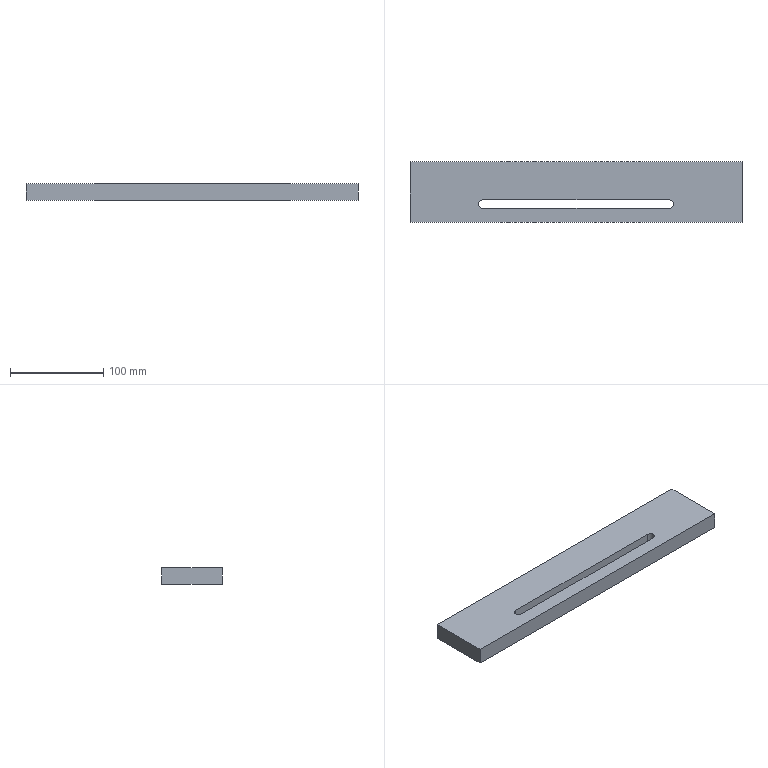Part | STEP file | Superstructure_1 | 1 solid | 10 faces | box 356.5 x 65 x 18 mm | volume 383560 mm3 | plane 8 | cylinder 2 | commonest cylinder face diameters 9 x2
STEP:
#1=CARTESIAN_POINT('',(0.,0.,0.));
#2=DIRECTION('',(0.,0.,1.));
#3=DIRECTION('',(1.,0.,0.));
#4=AXIS2_PLACEMENT_3D('',#1,#2,#3);
#5=CARTESIAN_POINT('',(-178.25,32.5,9.));
#6=VERTEX_POINT('',#5);
#7=CARTESIAN_POINT('',(-178.25,-32.5,9.));
#8=VERTEX_POINT('',#7);
#9=CARTESIAN_POINT('',(-178.25,32.5,9.));
#10=DIRECTION('',(0.,-1.,0.));
#11=VECTOR('',#10,1.);
#12=LINE('',#9,#11);
#13=CARTESIAN_POINT('',(-178.25,32.5,9.));
#14=DIRECTION('',(1.,0.,0.));
#15=DIRECTION('',(0.,0.,-1.));
#16=AXIS2_PLACEMENT_3D('',#13,#14,#15);
#17=PLANE('',#16);
#18=CARTESIAN_POINT('',(0.,0.));
#19=DIRECTION('',(0.,-1.));
#20=VECTOR('',#19,1.);
#21=LINE('',#18,#20);
#22=(GEOMETRIC_REPRESENTATION_CONTEXT(2)PARAMETRIC_REPRESENTATION_CONTEXT()REPRESENTATION_CONTEXT('',''));
#23=DEFINITIONAL_REPRESENTATION('',(#21),#22);
#24=PCURVE('',#17,#23);
#25=CARTESIAN_POINT('',(178.25,32.5,9.));
#26=DIRECTION('',(0.,0.,-1.));
#27=DIRECTION('',(-1.,0.,0.));
#28=AXIS2_PLACEMENT_3D('',#25,#26,#27);
#29=PLANE('',#28);
#30=CARTESIAN_POINT('',(356.5,0.));
#31=DIRECTION('',(0.,-1.));
#32=VECTOR('',#31,1.);
#33=LINE('',#30,#32);
#34=(GEOMETRIC_REPRESENTATION_CONTEXT(2)PARAMETRIC_REPRESENTATION_CONTEXT()REPRESENTATION_CONTEXT('',''));
#35=DEFINITIONAL_REPRESENTATION('',(#33),#34);
#36=PCURVE('',#29,#35);
#37=SURFACE_CURVE('',#12,(#24,#36),.PCURVE_S1.);
#38=EDGE_CURVE('',#6,#8,#37,.T.);
#39=ORIENTED_EDGE('',*,*,#38,.T.);
#40=CARTESIAN_POINT('',(-178.25,-32.5,-9.));
#41=VERTEX_POINT('',#40);
#42=CARTESIAN_POINT('',(-178.25,-32.5,9.));
#43=DIRECTION('',(0.,0.,-1.));
#44=VECTOR('',#43,1.);
#45=LINE('',#42,#44);
#46=CARTESIAN_POINT('',(0.,-65.));
#47=DIRECTION('',(1.,0.));
#48=VECTOR('',#47,1.);
#49=LINE('',#46,#48);
#50=(GEOMETRIC_REPRESENTATION_CONTEXT(2)PARAMETRIC_REPRESENTATION_CONTEXT()REPRESENTATION_CONTEXT('',''));
#51=DEFINITIONAL_REPRESENTATION('',(#49),#50);
#52=PCURVE('',#17,#51);
#53=CARTESIAN_POINT('',(0.,-32.5,0.));
#54=DIRECTION('',(0.,1.,0.));
#55=DIRECTION('',(0.,0.,1.));
#56=AXIS2_PLACEMENT_3D('',#53,#54,#55);
#57=PLANE('',#56);
#58=CARTESIAN_POINT('',(9.,-178.25));
#59=DIRECTION('',(-1.,0.));
#60=VECTOR('',#59,1.);
#61=LINE('',#58,#60);
#62=(GEOMETRIC_REPRESENTATION_CONTEXT(2)PARAMETRIC_REPRESENTATION_CONTEXT()REPRESENTATION_CONTEXT('',''));
#63=DEFINITIONAL_REPRESENTATION('',(#61),#62);
#64=PCURVE('',#57,#63);
#65=SURFACE_CURVE('',#45,(#52,#64),.PCURVE_S1.);
#66=EDGE_CURVE('',#8,#41,#65,.T.);
#67=ORIENTED_EDGE('',*,*,#66,.T.);
#68=CARTESIAN_POINT('',(-178.25,32.5,-9.));
#69=VERTEX_POINT('',#68);
#70=CARTESIAN_POINT('',(-178.25,32.5,-9.));
#71=DIRECTION('',(0.,-1.,0.));
#72=VECTOR('',#71,1.);
#73=LINE('',#70,#72);
#74=CARTESIAN_POINT('',(18.,0.));
#75=DIRECTION('',(0.,-1.));
#76=VECTOR('',#75,1.);
#77=LINE('',#74,#76);
#78=(GEOMETRIC_REPRESENTATION_CONTEXT(2)PARAMETRIC_REPRESENTATION_CONTEXT()REPRESENTATION_CONTEXT('',''));
#79=DEFINITIONAL_REPRESENTATION('',(#77),#78);
#80=PCURVE('',#17,#79);
#81=CARTESIAN_POINT('',(-178.25,32.5,-9.));
#82=DIRECTION('',(0.,0.,1.));
#83=DIRECTION('',(1.,0.,0.));
#84=AXIS2_PLACEMENT_3D('',#81,#82,#83);
#85=PLANE('',#84);
#86=CARTESIAN_POINT('',(0.,0.));
#87=DIRECTION('',(0.,-1.));
#88=VECTOR('',#87,1.);
#89=LINE('',#86,#88);
#90=(GEOMETRIC_REPRESENTATION_CONTEXT(2)PARAMETRIC_REPRESENTATION_CONTEXT()REPRESENTATION_CONTEXT('',''));
#91=DEFINITIONAL_REPRESENTATION('',(#89),#90);
#92=PCURVE('',#85,#91);
#93=SURFACE_CURVE('',#73,(#80,#92),.PCURVE_S1.);
#94=EDGE_CURVE('',#69,#41,#93,.T.);
#95=ORIENTED_EDGE('',*,*,#94,.F.);
#96=CARTESIAN_POINT('',(-178.25,32.5,9.));
#97=DIRECTION('',(0.,0.,-1.));
#98=VECTOR('',#97,1.);
#99=LINE('',#96,#98);
#100=CARTESIAN_POINT('',(0.,0.));
#101=DIRECTION('',(1.,0.));
#102=VECTOR('',#101,1.);
#103=LINE('',#100,#102);
#104=(GEOMETRIC_REPRESENTATION_CONTEXT(2)PARAMETRIC_REPRESENTATION_CONTEXT()REPRESENTATION_CONTEXT('',''));
#105=DEFINITIONAL_REPRESENTATION('',(#103),#104);
#106=PCURVE('',#17,#105);
#107=CARTESIAN_POINT('',(0.,32.5,0.));
#108=DIRECTION('',(0.,1.,0.));
#109=DIRECTION('',(0.,0.,1.));
#110=AXIS2_PLACEMENT_3D('',#107,#108,#109);
#111=PLANE('',#110);
#112=CARTESIAN_POINT('',(9.,-178.25));
#113=DIRECTION('',(-1.,0.));
#114=VECTOR('',#113,1.);
#115=LINE('',#112,#114);
#116=(GEOMETRIC_REPRESENTATION_CONTEXT(2)PARAMETRIC_REPRESENTATION_CONTEXT()REPRESENTATION_CONTEXT('',''));
#117=DEFINITIONAL_REPRESENTATION('',(#115),#116);
#118=PCURVE('',#111,#117);
#119=SURFACE_CURVE('',#99,(#106,#118),.PCURVE_S1.);
#120=EDGE_CURVE('',#6,#69,#119,.T.);
#121=ORIENTED_EDGE('',*,*,#120,.F.);
#122=EDGE_LOOP('',(#39,#67,#95,#121));
#123=FACE_BOUND('',#122,.F.);
#124=ADVANCED_FACE('',(#123),#17,.F.);
#125=CARTESIAN_POINT('',(178.25,32.5,9.));
#126=VERTEX_POINT('',#125);
#127=CARTESIAN_POINT('',(178.25,-32.5,9.));
#128=VERTEX_POINT('',#127);
#129=CARTESIAN_POINT('',(178.25,32.5,9.));
#130=DIRECTION('',(0.,-1.,0.));
#131=VECTOR('',#130,1.);
#132=LINE('',#129,#131);
#133=CARTESIAN_POINT('',(0.,0.));
#134=DIRECTION('',(0.,-1.));
#135=VECTOR('',#134,1.);
#136=LINE('',#133,#135);
#137=(GEOMETRIC_REPRESENTATION_CONTEXT(2)PARAMETRIC_REPRESENTATION_CONTEXT()REPRESENTATION_CONTEXT('',''));
#138=DEFINITIONAL_REPRESENTATION('',(#136),#137);
#139=PCURVE('',#29,#138);
#140=CARTESIAN_POINT('',(178.25,32.5,-9.));
#141=DIRECTION('',(-1.,0.,0.));
#142=DIRECTION('',(0.,0.,1.));
#143=AXIS2_PLACEMENT_3D('',#140,#141,#142);
#144=PLANE('',#143);
#145=CARTESIAN_POINT('',(18.,0.));
#146=DIRECTION('',(0.,-1.));
#147=VECTOR('',#146,1.);
#148=LINE('',#145,#147);
#149=(GEOMETRIC_REPRESENTATION_CONTEXT(2)PARAMETRIC_REPRESENTATION_CONTEXT()REPRESENTATION_CONTEXT('',''));
#150=DEFINITIONAL_REPRESENTATION('',(#148),#149);
#151=PCURVE('',#144,#150);
#152=SURFACE_CURVE('',#132,(#139,#151),.PCURVE_S1.);
#153=EDGE_CURVE('',#126,#128,#152,.T.);
#154=ORIENTED_EDGE('',*,*,#153,.T.);
#155=CARTESIAN_POINT('',(178.25,-32.5,9.));
#156=DIRECTION('',(-1.,0.,0.));
#157=VECTOR('',#156,1.);
#158=LINE('',#155,#157);
#159=CARTESIAN_POINT('',(0.,-65.));
#160=DIRECTION('',(1.,0.));
#161=VECTOR('',#160,1.);
#162=LINE('',#159,#161);
#163=(GEOMETRIC_REPRESENTATION_CONTEXT(2)PARAMETRIC_REPRESENTATION_CONTEXT()REPRESENTATION_CONTEXT('',''));
#164=DEFINITIONAL_REPRESENTATION('',(#162),#163);
#165=PCURVE('',#29,#164);
#166=CARTESIAN_POINT('',(9.,178.25));
#167=DIRECTION('',(0.,-1.));
#168=VECTOR('',#167,1.);
#169=LINE('',#166,#168);
#170=(GEOMETRIC_REPRESENTATION_CONTEXT(2)PARAMETRIC_REPRESENTATION_CONTEXT()REPRESENTATION_CONTEXT('',''));
#171=DEFINITIONAL_REPRESENTATION('',(#169),#170);
#172=PCURVE('',#57,#171);
#173=SURFACE_CURVE('',#158,(#165,#172),.PCURVE_S1.);
#174=EDGE_CURVE('',#128,#8,#173,.T.);
#175=ORIENTED_EDGE('',*,*,#174,.T.);
#176=ORIENTED_EDGE('',*,*,#38,.F.);
#177=CARTESIAN_POINT('',(178.25,32.5,9.));
#178=DIRECTION('',(-1.,0.,0.));
#179=VECTOR('',#178,1.);
#180=LINE('',#177,#179);
#181=CARTESIAN_POINT('',(0.,0.));
#182=DIRECTION('',(1.,0.));
#183=VECTOR('',#182,1.);
#184=LINE('',#181,#183);
#185=(GEOMETRIC_REPRESENTATION_CONTEXT(2)PARAMETRIC_REPRESENTATION_CONTEXT()REPRESENTATION_CONTEXT('',''));
#186=DEFINITIONAL_REPRESENTATION('',(#184),#185);
#187=PCURVE('',#29,#186);
#188=CARTESIAN_POINT('',(9.,178.25));
#189=DIRECTION('',(0.,-1.));
#190=VECTOR('',#189,1.);
#191=LINE('',#188,#190);
#192=(GEOMETRIC_REPRESENTATION_CONTEXT(2)PARAMETRIC_REPRESENTATION_CONTEXT()REPRESENTATION_CONTEXT('',''));
#193=DEFINITIONAL_REPRESENTATION('',(#191),#192);
#194=PCURVE('',#111,#193);
#195=SURFACE_CURVE('',#180,(#187,#194),.PCURVE_S1.);
#196=EDGE_CURVE('',#126,#6,#195,.T.);
#197=ORIENTED_EDGE('',*,*,#196,.F.);
#198=EDGE_LOOP('',(#154,#175,#176,#197));
#199=FACE_BOUND('',#198,.F.);
#200=CARTESIAN_POINT('',(100.,-8.5,9.));
#201=VERTEX_POINT('',#200);
#202=CARTESIAN_POINT('',(-100.,-8.5,9.));
#203=VERTEX_POINT('',#202);
#204=CARTESIAN_POINT('',(39.125,-8.5,9.));
#205=DIRECTION('',(-1.,0.,0.));
#206=VECTOR('',#205,1.);
#207=LINE('',#204,#206);
#208=CARTESIAN_POINT('',(139.125,-41.));
#209=DIRECTION('',(1.,0.));
#210=VECTOR('',#209,1.);
#211=LINE('',#208,#210);
#212=(GEOMETRIC_REPRESENTATION_CONTEXT(2)PARAMETRIC_REPRESENTATION_CONTEXT()REPRESENTATION_CONTEXT('',''));
#213=DEFINITIONAL_REPRESENTATION('',(#211),#212);
#214=PCURVE('',#29,#213);
#215=CARTESIAN_POINT('',(-100.,-8.5,15.));
#216=DIRECTION('',(0.,-1.,0.));
#217=DIRECTION('',(1.,0.,0.));
#218=AXIS2_PLACEMENT_3D('',#215,#216,#217);
#219=PLANE('',#218);
#220=CARTESIAN_POINT('',(139.125,-6.));
#221=DIRECTION('',(-1.,0.));
#222=VECTOR('',#221,1.);
#223=LINE('',#220,#222);
#224=(GEOMETRIC_REPRESENTATION_CONTEXT(2)PARAMETRIC_REPRESENTATION_CONTEXT()REPRESENTATION_CONTEXT('',''));
#225=DEFINITIONAL_REPRESENTATION('',(#223),#224);
#226=PCURVE('',#219,#225);
#227=SURFACE_CURVE('',#207,(#214,#226),.PCURVE_S1.);
#228=EDGE_CURVE('',#201,#203,#227,.T.);
#229=ORIENTED_EDGE('',*,*,#228,.T.);
#230=CARTESIAN_POINT('',(-100.,-17.5,9.));
#231=VERTEX_POINT('',#230);
#232=CARTESIAN_POINT('',(-100.,-13.,9.));
#233=DIRECTION('',(0.,0.,1.));
#234=DIRECTION('',(1.,0.,0.));
#235=AXIS2_PLACEMENT_3D('',#232,#233,#234);
#236=CIRCLE('',#235,4.5);
#237=CARTESIAN_POINT('',(273.75,-45.5));
#238=CARTESIAN_POINT('',(273.75,-37.706));
#239=CARTESIAN_POINT('',(280.5,-41.603));
#240=CARTESIAN_POINT('',(287.25,-45.5));
#241=CARTESIAN_POINT('',(280.5,-49.397));
#242=CARTESIAN_POINT('',(273.75,-53.294));
#243=CARTESIAN_POINT('',(273.75,-45.5));
#244=(BOUNDED_CURVE()B_SPLINE_CURVE(2,(#237,#238,#239,#240,#241,#242,#243),.UNSPECIFIED.,.T.,.F.)B_SPLINE_CURVE_WITH_KNOTS((1,2,2,2,2,1),(-2.094,0.,2.094,4.189,6.283,8.378),.UNSPECIFIED.)CURVE()GEOMETRIC_REPRESENTATION_ITEM()RATIONAL_B_SPLINE_CURVE((1.,0.5,1.,0.5,1.,0.5,1.))REPRESENTATION_ITEM(''));
#245=(GEOMETRIC_REPRESENTATION_CONTEXT(2)PARAMETRIC_REPRESENTATION_CONTEXT()REPRESENTATION_CONTEXT('',''));
#246=DEFINITIONAL_REPRESENTATION('',(#244),#245);
#247=PCURVE('',#29,#246);
#248=CARTESIAN_POINT('',(-100.,-13.,15.));
#249=DIRECTION('',(0.,0.,1.));
#250=DIRECTION('',(1.,0.,0.));
#251=AXIS2_PLACEMENT_3D('',#248,#249,#250);
#252=CYLINDRICAL_SURFACE('',#251,4.5);
#253=CARTESIAN_POINT('',(0.,-6.));
#254=DIRECTION('',(1.,0.));
#255=VECTOR('',#254,1.);
#256=LINE('',#253,#255);
#257=(GEOMETRIC_REPRESENTATION_CONTEXT(2)PARAMETRIC_REPRESENTATION_CONTEXT()REPRESENTATION_CONTEXT('',''));
#258=DEFINITIONAL_REPRESENTATION('',(#256),#257);
#259=PCURVE('',#252,#258);
#260=SURFACE_CURVE('',#236,(#247,#259),.PCURVE_S1.);
#261=EDGE_CURVE('',#203,#231,#260,.T.);
#262=ORIENTED_EDGE('',*,*,#261,.T.);
#263=CARTESIAN_POINT('',(100.,-17.5,9.));
#264=VERTEX_POINT('',#263);
#265=CARTESIAN_POINT('',(39.125,-17.5,9.));
#266=DIRECTION('',(-1.,0.,0.));
#267=VECTOR('',#266,1.);
#268=LINE('',#265,#267);
#269=CARTESIAN_POINT('',(139.125,-50.));
#270=DIRECTION('',(1.,0.));
#271=VECTOR('',#270,1.);
#272=LINE('',#269,#271);
#273=(GEOMETRIC_REPRESENTATION_CONTEXT(2)PARAMETRIC_REPRESENTATION_CONTEXT()REPRESENTATION_CONTEXT('',''));
#274=DEFINITIONAL_REPRESENTATION('',(#272),#273);
#275=PCURVE('',#29,#274);
#276=CARTESIAN_POINT('',(-100.,-17.5,15.));
#277=DIRECTION('',(0.,-1.,0.));
#278=DIRECTION('',(1.,0.,0.));
#279=AXIS2_PLACEMENT_3D('',#276,#277,#278);
#280=PLANE('',#279);
#281=CARTESIAN_POINT('',(139.125,-6.));
#282=DIRECTION('',(-1.,0.));
#283=VECTOR('',#282,1.);
#284=LINE('',#281,#283);
#285=(GEOMETRIC_REPRESENTATION_CONTEXT(2)PARAMETRIC_REPRESENTATION_CONTEXT()REPRESENTATION_CONTEXT('',''));
#286=DEFINITIONAL_REPRESENTATION('',(#284),#285);
#287=PCURVE('',#280,#286);
#288=SURFACE_CURVE('',#268,(#275,#287),.PCURVE_S1.);
#289=EDGE_CURVE('',#264,#231,#288,.T.);
#290=ORIENTED_EDGE('',*,*,#289,.F.);
#291=CARTESIAN_POINT('',(100.,-13.,9.));
#292=DIRECTION('',(0.,0.,1.));
#293=DIRECTION('',(1.,0.,0.));
#294=AXIS2_PLACEMENT_3D('',#291,#292,#293);
#295=CIRCLE('',#294,4.5);
#296=CARTESIAN_POINT('',(73.75,-45.5));
#297=CARTESIAN_POINT('',(73.75,-37.706));
#298=CARTESIAN_POINT('',(80.5,-41.603));
#299=CARTESIAN_POINT('',(87.25,-45.5));
#300=CARTESIAN_POINT('',(80.5,-49.397));
#301=CARTESIAN_POINT('',(73.75,-53.294));
#302=CARTESIAN_POINT('',(73.75,-45.5));
#303=(BOUNDED_CURVE()B_SPLINE_CURVE(2,(#296,#297,#298,#299,#300,#301,#302),.UNSPECIFIED.,.T.,.F.)B_SPLINE_CURVE_WITH_KNOTS((1,2,2,2,2,1),(-2.094,0.,2.094,4.189,6.283,8.378),.UNSPECIFIED.)CURVE()GEOMETRIC_REPRESENTATION_ITEM()RATIONAL_B_SPLINE_CURVE((1.,0.5,1.,0.5,1.,0.5,1.))REPRESENTATION_ITEM(''));
#304=(GEOMETRIC_REPRESENTATION_CONTEXT(2)PARAMETRIC_REPRESENTATION_CONTEXT()REPRESENTATION_CONTEXT('',''));
#305=DEFINITIONAL_REPRESENTATION('',(#303),#304);
#306=PCURVE('',#29,#305);
#307=CARTESIAN_POINT('',(100.,-13.,15.));
#308=DIRECTION('',(0.,0.,1.));
#309=DIRECTION('',(1.,0.,0.));
#310=AXIS2_PLACEMENT_3D('',#307,#308,#309);
#311=CYLINDRICAL_SURFACE('',#310,4.5);
#312=CARTESIAN_POINT('',(0.,-6.));
#313=DIRECTION('',(1.,0.));
#314=VECTOR('',#313,1.);
#315=LINE('',#312,#314);
#316=(GEOMETRIC_REPRESENTATION_CONTEXT(2)PARAMETRIC_REPRESENTATION_CONTEXT()REPRESENTATION_CONTEXT('',''));
#317=DEFINITIONAL_REPRESENTATION('',(#315),#316);
#318=PCURVE('',#311,#317);
#319=SURFACE_CURVE('',#295,(#306,#318),.PCURVE_S1.);
#320=EDGE_CURVE('',#264,#201,#319,.T.);
#321=ORIENTED_EDGE('',*,*,#320,.T.);
#322=EDGE_LOOP('',(#229,#262,#290,#321));
#323=FACE_BOUND('',#322,.F.);
#324=ADVANCED_FACE('',(#199,#323),#29,.F.);
#325=ORIENTED_EDGE('',*,*,#94,.T.);
#326=CARTESIAN_POINT('',(178.25,-32.5,-9.));
#327=VERTEX_POINT('',#326);
#328=CARTESIAN_POINT('',(-178.25,-32.5,-9.));
#329=DIRECTION('',(1.,0.,0.));
#330=VECTOR('',#329,1.);
#331=LINE('',#328,#330);
#332=CARTESIAN_POINT('',(0.,-65.));
#333=DIRECTION('',(1.,0.));
#334=VECTOR('',#333,1.);
#335=LINE('',#332,#334);
#336=(GEOMETRIC_REPRESENTATION_CONTEXT(2)PARAMETRIC_REPRESENTATION_CONTEXT()REPRESENTATION_CONTEXT('',''));
#337=DEFINITIONAL_REPRESENTATION('',(#335),#336);
#338=PCURVE('',#85,#337);
#339=CARTESIAN_POINT('',(-9.,-178.25));
#340=DIRECTION('',(0.,1.));
#341=VECTOR('',#340,1.);
#342=LINE('',#339,#341);
#343=(GEOMETRIC_REPRESENTATION_CONTEXT(2)PARAMETRIC_REPRESENTATION_CONTEXT()REPRESENTATION_CONTEXT('',''));
#344=DEFINITIONAL_REPRESENTATION('',(#342),#343);
#345=PCURVE('',#57,#344);
#346=SURFACE_CURVE('',#331,(#338,#345),.PCURVE_S1.);
#347=EDGE_CURVE('',#41,#327,#346,.T.);
#348=ORIENTED_EDGE('',*,*,#347,.T.);
#349=CARTESIAN_POINT('',(178.25,32.5,-9.));
#350=VERTEX_POINT('',#349);
#351=CARTESIAN_POINT('',(178.25,32.5,-9.));
#352=DIRECTION('',(0.,-1.,0.));
#353=VECTOR('',#352,1.);
#354=LINE('',#351,#353);
#355=CARTESIAN_POINT('',(356.5,0.));
#356=DIRECTION('',(0.,-1.));
#357=VECTOR('',#356,1.);
#358=LINE('',#355,#357);
#359=(GEOMETRIC_REPRESENTATION_CONTEXT(2)PARAMETRIC_REPRESENTATION_CONTEXT()REPRESENTATION_CONTEXT('',''));
#360=DEFINITIONAL_REPRESENTATION('',(#358),#359);
#361=PCURVE('',#85,#360);
#362=CARTESIAN_POINT('',(0.,0.));
#363=DIRECTION('',(0.,-1.));
#364=VECTOR('',#363,1.);
#365=LINE('',#362,#364);
#366=(GEOMETRIC_REPRESENTATION_CONTEXT(2)PARAMETRIC_REPRESENTATION_CONTEXT()REPRESENTATION_CONTEXT('',''));
#367=DEFINITIONAL_REPRESENTATION('',(#365),#366);
#368=PCURVE('',#144,#367);
#369=SURFACE_CURVE('',#354,(#361,#368),.PCURVE_S1.);
#370=EDGE_CURVE('',#350,#327,#369,.T.);
#371=ORIENTED_EDGE('',*,*,#370,.F.);
#372=CARTESIAN_POINT('',(-178.25,32.5,-9.));
#373=DIRECTION('',(1.,0.,0.));
#374=VECTOR('',#373,1.);
#375=LINE('',#372,#374);
#376=CARTESIAN_POINT('',(0.,0.));
#377=DIRECTION('',(1.,0.));
#378=VECTOR('',#377,1.);
#379=LINE('',#376,#378);
#380=(GEOMETRIC_REPRESENTATION_CONTEXT(2)PARAMETRIC_REPRESENTATION_CONTEXT()REPRESENTATION_CONTEXT('',''));
#381=DEFINITIONAL_REPRESENTATION('',(#379),#380);
#382=PCURVE('',#85,#381);
#383=CARTESIAN_POINT('',(-9.,-178.25));
#384=DIRECTION('',(0.,1.));
#385=VECTOR('',#384,1.);
#386=LINE('',#383,#385);
#387=(GEOMETRIC_REPRESENTATION_CONTEXT(2)PARAMETRIC_REPRESENTATION_CONTEXT()REPRESENTATION_CONTEXT('',''));
#388=DEFINITIONAL_REPRESENTATION('',(#386),#387);
#389=PCURVE('',#111,#388);
#390=SURFACE_CURVE('',#375,(#382,#389),.PCURVE_S1.);
#391=EDGE_CURVE('',#69,#350,#390,.T.);
#392=ORIENTED_EDGE('',*,*,#391,.F.);
#393=EDGE_LOOP('',(#325,#348,#371,#392));
#394=FACE_BOUND('',#393,.F.);
#395=CARTESIAN_POINT('',(-100.,-8.5,-9.));
#396=VERTEX_POINT('',#395);
#397=CARTESIAN_POINT('',(-100.,-17.5,-9.));
#398=VERTEX_POINT('',#397);
#399=CARTESIAN_POINT('',(-100.,-13.,-9.));
#400=DIRECTION('',(0.,0.,1.));
#401=DIRECTION('',(1.,0.,0.));
#402=AXIS2_PLACEMENT_3D('',#399,#400,#401);
#403=CIRCLE('',#402,4.5);
#404=CARTESIAN_POINT('',(78.25,-45.5));
#405=DIRECTION('',(1.,0.));
#406=AXIS2_PLACEMENT_2D('',#404,#405);
#407=CIRCLE('',#406,4.5);
#408=(GEOMETRIC_REPRESENTATION_CONTEXT(2)PARAMETRIC_REPRESENTATION_CONTEXT()REPRESENTATION_CONTEXT('',''));
#409=DEFINITIONAL_REPRESENTATION('',(#407),#408);
#410=PCURVE('',#85,#409);
#411=CARTESIAN_POINT('',(0.,-24.));
#412=DIRECTION('',(1.,0.));
#413=VECTOR('',#412,1.);
#414=LINE('',#411,#413);
#415=(GEOMETRIC_REPRESENTATION_CONTEXT(2)PARAMETRIC_REPRESENTATION_CONTEXT()REPRESENTATION_CONTEXT('',''));
#416=DEFINITIONAL_REPRESENTATION('',(#414),#415);
#417=PCURVE('',#252,#416);
#418=SURFACE_CURVE('',#403,(#410,#417),.PCURVE_S1.);
#419=EDGE_CURVE('',#396,#398,#418,.T.);
#420=ORIENTED_EDGE('',*,*,#419,.F.);
#421=CARTESIAN_POINT('',(100.,-8.5,-9.));
#422=VERTEX_POINT('',#421);
#423=CARTESIAN_POINT('',(-139.125,-8.5,-9.));
#424=DIRECTION('',(1.,0.,0.));
#425=VECTOR('',#424,1.);
#426=LINE('',#423,#425);
#427=CARTESIAN_POINT('',(39.125,-41.));
#428=DIRECTION('',(1.,0.));
#429=VECTOR('',#428,1.);
#430=LINE('',#427,#429);
#431=(GEOMETRIC_REPRESENTATION_CONTEXT(2)PARAMETRIC_REPRESENTATION_CONTEXT()REPRESENTATION_CONTEXT('',''));
#432=DEFINITIONAL_REPRESENTATION('',(#430),#431);
#433=PCURVE('',#85,#432);
#434=CARTESIAN_POINT('',(-39.125,-24.));
#435=DIRECTION('',(1.,0.));
#436=VECTOR('',#435,1.);
#437=LINE('',#434,#436);
#438=(GEOMETRIC_REPRESENTATION_CONTEXT(2)PARAMETRIC_REPRESENTATION_CONTEXT()REPRESENTATION_CONTEXT('',''));
#439=DEFINITIONAL_REPRESENTATION('',(#437),#438);
#440=PCURVE('',#219,#439);
#441=SURFACE_CURVE('',#426,(#433,#440),.PCURVE_S1.);
#442=EDGE_CURVE('',#396,#422,#441,.T.);
#443=ORIENTED_EDGE('',*,*,#442,.T.);
#444=CARTESIAN_POINT('',(100.,-17.5,-9.));
#445=VERTEX_POINT('',#444);
#446=CARTESIAN_POINT('',(100.,-13.,-9.));
#447=DIRECTION('',(0.,0.,1.));
#448=DIRECTION('',(1.,0.,0.));
#449=AXIS2_PLACEMENT_3D('',#446,#447,#448);
#450=CIRCLE('',#449,4.5);
#451=CARTESIAN_POINT('',(278.25,-45.5));
#452=DIRECTION('',(1.,0.));
#453=AXIS2_PLACEMENT_2D('',#451,#452);
#454=CIRCLE('',#453,4.5);
#455=(GEOMETRIC_REPRESENTATION_CONTEXT(2)PARAMETRIC_REPRESENTATION_CONTEXT()REPRESENTATION_CONTEXT('',''));
#456=DEFINITIONAL_REPRESENTATION('',(#454),#455);
#457=PCURVE('',#85,#456);
#458=CARTESIAN_POINT('',(0.,-24.));
#459=DIRECTION('',(1.,0.));
#460=VECTOR('',#459,1.);
#461=LINE('',#458,#460);
#462=(GEOMETRIC_REPRESENTATION_CONTEXT(2)PARAMETRIC_REPRESENTATION_CONTEXT()REPRESENTATION_CONTEXT('',''));
#463=DEFINITIONAL_REPRESENTATION('',(#461),#462);
#464=PCURVE('',#311,#463);
#465=SURFACE_CURVE('',#450,(#457,#464),.PCURVE_S1.);
#466=EDGE_CURVE('',#445,#422,#465,.T.);
#467=ORIENTED_EDGE('',*,*,#466,.F.);
#468=CARTESIAN_POINT('',(-139.125,-17.5,-9.));
#469=DIRECTION('',(1.,0.,0.));
#470=VECTOR('',#469,1.);
#471=LINE('',#468,#470);
#472=CARTESIAN_POINT('',(39.125,-50.));
#473=DIRECTION('',(1.,0.));
#474=VECTOR('',#473,1.);
#475=LINE('',#472,#474);
#476=(GEOMETRIC_REPRESENTATION_CONTEXT(2)PARAMETRIC_REPRESENTATION_CONTEXT()REPRESENTATION_CONTEXT('',''));
#477=DEFINITIONAL_REPRESENTATION('',(#475),#476);
#478=PCURVE('',#85,#477);
#479=CARTESIAN_POINT('',(-39.125,-24.));
#480=DIRECTION('',(1.,0.));
#481=VECTOR('',#480,1.);
#482=LINE('',#479,#481);
#483=(GEOMETRIC_REPRESENTATION_CONTEXT(2)PARAMETRIC_REPRESENTATION_CONTEXT()REPRESENTATION_CONTEXT('',''));
#484=DEFINITIONAL_REPRESENTATION('',(#482),#483);
#485=PCURVE('',#280,#484);
#486=SURFACE_CURVE('',#471,(#478,#485),.PCURVE_S1.);
#487=EDGE_CURVE('',#398,#445,#486,.T.);
#488=ORIENTED_EDGE('',*,*,#487,.F.);
#489=EDGE_LOOP('',(#420,#443,#467,#488));
#490=FACE_BOUND('',#489,.F.);
#491=ADVANCED_FACE('',(#394,#490),#85,.F.);
#492=ORIENTED_EDGE('',*,*,#120,.T.);
#493=ORIENTED_EDGE('',*,*,#391,.T.);
#494=CARTESIAN_POINT('',(178.25,32.5,-9.));
#495=DIRECTION('',(0.,0.,1.));
#496=VECTOR('',#495,1.);
#497=LINE('',#494,#496);
#498=CARTESIAN_POINT('',(-9.,178.25));
#499=DIRECTION('',(1.,0.));
#500=VECTOR('',#499,1.);
#501=LINE('',#498,#500);
#502=(GEOMETRIC_REPRESENTATION_CONTEXT(2)PARAMETRIC_REPRESENTATION_CONTEXT()REPRESENTATION_CONTEXT('',''));
#503=DEFINITIONAL_REPRESENTATION('',(#501),#502);
#504=PCURVE('',#111,#503);
#505=CARTESIAN_POINT('',(0.,0.));
#506=DIRECTION('',(1.,0.));
#507=VECTOR('',#506,1.);
#508=LINE('',#505,#507);
#509=(GEOMETRIC_REPRESENTATION_CONTEXT(2)PARAMETRIC_REPRESENTATION_CONTEXT()REPRESENTATION_CONTEXT('',''));
#510=DEFINITIONAL_REPRESENTATION('',(#508),#509);
#511=PCURVE('',#144,#510);
#512=SURFACE_CURVE('',#497,(#504,#511),.PCURVE_S1.);
#513=EDGE_CURVE('',#350,#126,#512,.T.);
#514=ORIENTED_EDGE('',*,*,#513,.T.);
#515=ORIENTED_EDGE('',*,*,#196,.T.);
#516=EDGE_LOOP('',(#492,#493,#514,#515));
#517=FACE_BOUND('',#516,.F.);
#518=ADVANCED_FACE('',(#517),#111,.T.);
#519=ORIENTED_EDGE('',*,*,#66,.T.);
#520=ORIENTED_EDGE('',*,*,#347,.T.);
#521=CARTESIAN_POINT('',(178.25,-32.5,-9.));
#522=DIRECTION('',(0.,0.,1.));
#523=VECTOR('',#522,1.);
#524=LINE('',#521,#523);
#525=CARTESIAN_POINT('',(-9.,178.25));
#526=DIRECTION('',(1.,0.));
#527=VECTOR('',#526,1.);
#528=LINE('',#525,#527);
#529=(GEOMETRIC_REPRESENTATION_CONTEXT(2)PARAMETRIC_REPRESENTATION_CONTEXT()REPRESENTATION_CONTEXT('',''));
#530=DEFINITIONAL_REPRESENTATION('',(#528),#529);
#531=PCURVE('',#57,#530);
#532=CARTESIAN_POINT('',(0.,-65.));
#533=DIRECTION('',(1.,0.));
#534=VECTOR('',#533,1.);
#535=LINE('',#532,#534);
#536=(GEOMETRIC_REPRESENTATION_CONTEXT(2)PARAMETRIC_REPRESENTATION_CONTEXT()REPRESENTATION_CONTEXT('',''));
#537=DEFINITIONAL_REPRESENTATION('',(#535),#536);
#538=PCURVE('',#144,#537);
#539=SURFACE_CURVE('',#524,(#531,#538),.PCURVE_S1.);
#540=EDGE_CURVE('',#327,#128,#539,.T.);
#541=ORIENTED_EDGE('',*,*,#540,.T.);
#542=ORIENTED_EDGE('',*,*,#174,.T.);
#543=EDGE_LOOP('',(#519,#520,#541,#542));
#544=FACE_BOUND('',#543,.T.);
#545=ADVANCED_FACE('',(#544),#57,.F.);
#546=ORIENTED_EDGE('',*,*,#370,.T.);
#547=ORIENTED_EDGE('',*,*,#540,.T.);
#548=ORIENTED_EDGE('',*,*,#153,.F.);
#549=ORIENTED_EDGE('',*,*,#513,.F.);
#550=EDGE_LOOP('',(#546,#547,#548,#549));
#551=FACE_BOUND('',#550,.F.);
#552=ADVANCED_FACE('',(#551),#144,.F.);
#553=ORIENTED_EDGE('',*,*,#228,.T.);
#554=CARTESIAN_POINT('',(-100.,-8.5,15.));
#555=DIRECTION('',(0.,0.,-1.));
#556=VECTOR('',#555,1.);
#557=LINE('',#554,#556);
#558=CARTESIAN_POINT('',(0.,0.));
#559=DIRECTION('',(0.,-1.));
#560=VECTOR('',#559,1.);
#561=LINE('',#558,#560);
#562=(GEOMETRIC_REPRESENTATION_CONTEXT(2)PARAMETRIC_REPRESENTATION_CONTEXT()REPRESENTATION_CONTEXT('',''));
#563=DEFINITIONAL_REPRESENTATION('',(#561),#562);
#564=PCURVE('',#219,#563);
#565=CARTESIAN_POINT('',(1.571,0.));
#566=DIRECTION('',(0.,-1.));
#567=VECTOR('',#566,1.);
#568=LINE('',#565,#567);
#569=(GEOMETRIC_REPRESENTATION_CONTEXT(2)PARAMETRIC_REPRESENTATION_CONTEXT()REPRESENTATION_CONTEXT('',''));
#570=DEFINITIONAL_REPRESENTATION('',(#568),#569);
#571=PCURVE('',#252,#570);
#572=SURFACE_CURVE('',#557,(#564,#571),.PCURVE_S1.);
#573=EDGE_CURVE('',#203,#396,#572,.T.);
#574=ORIENTED_EDGE('',*,*,#573,.T.);
#575=ORIENTED_EDGE('',*,*,#442,.T.);
#576=CARTESIAN_POINT('',(100.,-8.5,15.));
#577=DIRECTION('',(0.,0.,-1.));
#578=VECTOR('',#577,1.);
#579=LINE('',#576,#578);
#580=CARTESIAN_POINT('',(200.,0.));
#581=DIRECTION('',(0.,-1.));
#582=VECTOR('',#581,1.);
#583=LINE('',#580,#582);
#584=(GEOMETRIC_REPRESENTATION_CONTEXT(2)PARAMETRIC_REPRESENTATION_CONTEXT()REPRESENTATION_CONTEXT('',''));
#585=DEFINITIONAL_REPRESENTATION('',(#583),#584);
#586=PCURVE('',#219,#585);
#587=CARTESIAN_POINT('',(7.854,0.));
#588=DIRECTION('',(0.,-1.));
#589=VECTOR('',#588,1.);
#590=LINE('',#587,#589);
#591=(GEOMETRIC_REPRESENTATION_CONTEXT(2)PARAMETRIC_REPRESENTATION_CONTEXT()REPRESENTATION_CONTEXT('',''));
#592=DEFINITIONAL_REPRESENTATION('',(#590),#591);
#593=PCURVE('',#311,#592);
#594=SURFACE_CURVE('',#579,(#586,#593),.PCURVE_S1.);
#595=EDGE_CURVE('',#201,#422,#594,.T.);
#596=ORIENTED_EDGE('',*,*,#595,.F.);
#597=EDGE_LOOP('',(#553,#574,#575,#596));
#598=FACE_BOUND('',#597,.T.);
#599=ADVANCED_FACE('',(#598),#219,.T.);
#600=ORIENTED_EDGE('',*,*,#320,.F.);
#601=CARTESIAN_POINT('',(100.,-17.5,15.));
#602=DIRECTION('',(0.,0.,-1.));
#603=VECTOR('',#602,1.);
#604=LINE('',#601,#603);
#605=CARTESIAN_POINT('',(4.712,0.));
#606=DIRECTION('',(0.,-1.));
#607=VECTOR('',#606,1.);
#608=LINE('',#605,#607);
#609=(GEOMETRIC_REPRESENTATION_CONTEXT(2)PARAMETRIC_REPRESENTATION_CONTEXT()REPRESENTATION_CONTEXT('',''));
#610=DEFINITIONAL_REPRESENTATION('',(#608),#609);
#611=PCURVE('',#311,#610);
#612=CARTESIAN_POINT('',(200.,0.));
#613=DIRECTION('',(0.,-1.));
#614=VECTOR('',#613,1.);
#615=LINE('',#612,#614);
#616=(GEOMETRIC_REPRESENTATION_CONTEXT(2)PARAMETRIC_REPRESENTATION_CONTEXT()REPRESENTATION_CONTEXT('',''));
#617=DEFINITIONAL_REPRESENTATION('',(#615),#616);
#618=PCURVE('',#280,#617);
#619=SURFACE_CURVE('',#604,(#611,#618),.PCURVE_S1.);
#620=EDGE_CURVE('',#264,#445,#619,.T.);
#621=ORIENTED_EDGE('',*,*,#620,.T.);
#622=ORIENTED_EDGE('',*,*,#466,.T.);
#623=ORIENTED_EDGE('',*,*,#595,.F.);
#624=EDGE_LOOP('',(#600,#621,#622,#623));
#625=FACE_BOUND('',#624,.F.);
#626=ADVANCED_FACE('',(#625),#311,.F.);
#627=ORIENTED_EDGE('',*,*,#289,.T.);
#628=CARTESIAN_POINT('',(-100.,-17.5,15.));
#629=DIRECTION('',(0.,0.,-1.));
#630=VECTOR('',#629,1.);
#631=LINE('',#628,#630);
#632=CARTESIAN_POINT('',(0.,0.));
#633=DIRECTION('',(0.,-1.));
#634=VECTOR('',#633,1.);
#635=LINE('',#632,#634);
#636=(GEOMETRIC_REPRESENTATION_CONTEXT(2)PARAMETRIC_REPRESENTATION_CONTEXT()REPRESENTATION_CONTEXT('',''));
#637=DEFINITIONAL_REPRESENTATION('',(#635),#636);
#638=PCURVE('',#280,#637);
#639=CARTESIAN_POINT('',(4.712,0.));
#640=DIRECTION('',(0.,-1.));
#641=VECTOR('',#640,1.);
#642=LINE('',#639,#641);
#643=(GEOMETRIC_REPRESENTATION_CONTEXT(2)PARAMETRIC_REPRESENTATION_CONTEXT()REPRESENTATION_CONTEXT('',''));
#644=DEFINITIONAL_REPRESENTATION('',(#642),#643);
#645=PCURVE('',#252,#644);
#646=SURFACE_CURVE('',#631,(#638,#645),.PCURVE_S1.);
#647=EDGE_CURVE('',#231,#398,#646,.T.);
#648=ORIENTED_EDGE('',*,*,#647,.T.);
#649=ORIENTED_EDGE('',*,*,#487,.T.);
#650=ORIENTED_EDGE('',*,*,#620,.F.);
#651=EDGE_LOOP('',(#627,#648,#649,#650));
#652=FACE_BOUND('',#651,.F.);
#653=ADVANCED_FACE('',(#652),#280,.F.);
#654=ORIENTED_EDGE('',*,*,#261,.F.);
#655=ORIENTED_EDGE('',*,*,#573,.T.);
#656=ORIENTED_EDGE('',*,*,#419,.T.);
#657=ORIENTED_EDGE('',*,*,#647,.F.);
#658=EDGE_LOOP('',(#654,#655,#656,#657));
#659=FACE_BOUND('',#658,.F.);
#660=ADVANCED_FACE('',(#659),#252,.F.);
#661=CLOSED_SHELL('',(#124,#324,#491,#518,#545,#552,#599,#626,#653,#660));
#662=MANIFOLD_SOLID_BREP('',#661);
#663=(LENGTH_UNIT()NAMED_UNIT(*)SI_UNIT(.MILLI.,.METRE.));
#664=UNCERTAINTY_MEASURE_WITH_UNIT(LENGTH_MEASURE(0.0000001),#663,'','');
#665=(NAMED_UNIT(*)PLANE_ANGLE_UNIT()SI_UNIT($,.RADIAN.));
#666=(NAMED_UNIT(*)SI_UNIT($,.STERADIAN.)SOLID_ANGLE_UNIT());
#667=(GEOMETRIC_REPRESENTATION_CONTEXT(3)GLOBAL_UNCERTAINTY_ASSIGNED_CONTEXT((#664))GLOBAL_UNIT_ASSIGNED_CONTEXT((#663,#665,#666))REPRESENTATION_CONTEXT('',''));
#668=ADVANCED_BREP_SHAPE_REPRESENTATION('',(#4,#662),#667);